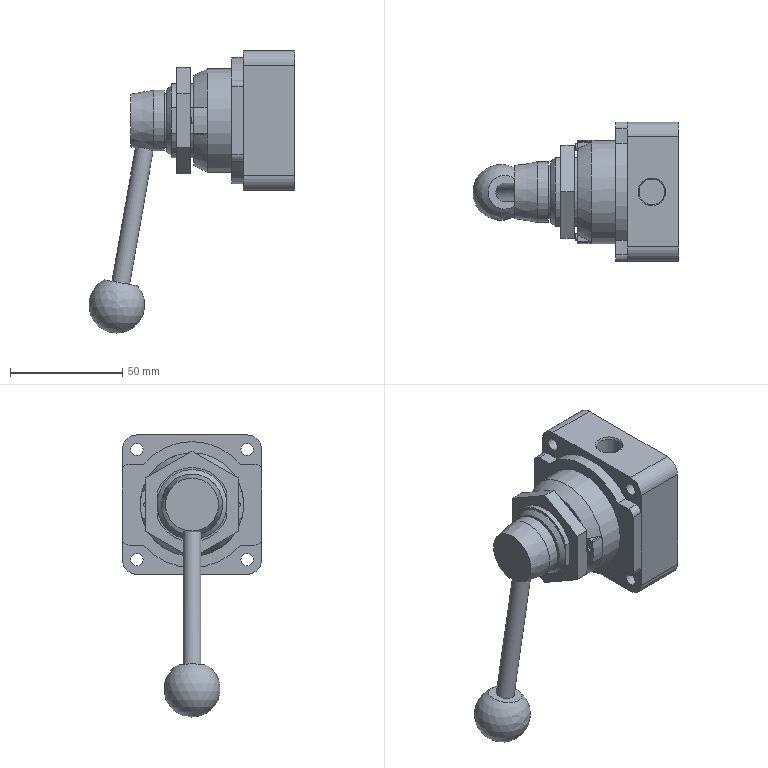Part | NX | features PARTBODY 2 | 1 solid | 86 faces | box 91.659 x 62 x 125.5 mm | volume 154933 mm3 | plane 42 | cylinder 36 | cone 7 | sphere 1 | commonest cylinder face diameters 1 x4 5.5 x4 6 x4 11.45 x4 13 x4 33 x4